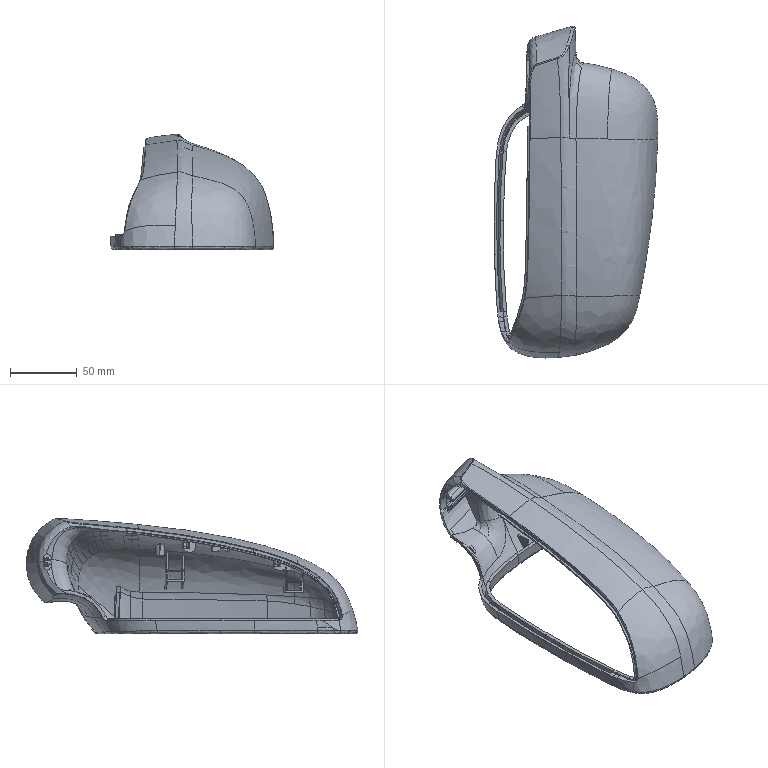Part | STEP file | 车灯-后视镜_id198_x_t | 1 solid | 575 faces | box 122.477 x 248.122 x 87.358 mm | volume 134816 mm3 | spline 361 | plane 207 | cylinder 7 | commonest cylinder face diameters 1.018 x2 7.035 x2 1.003 x1 5.624 x1 53.964 x1